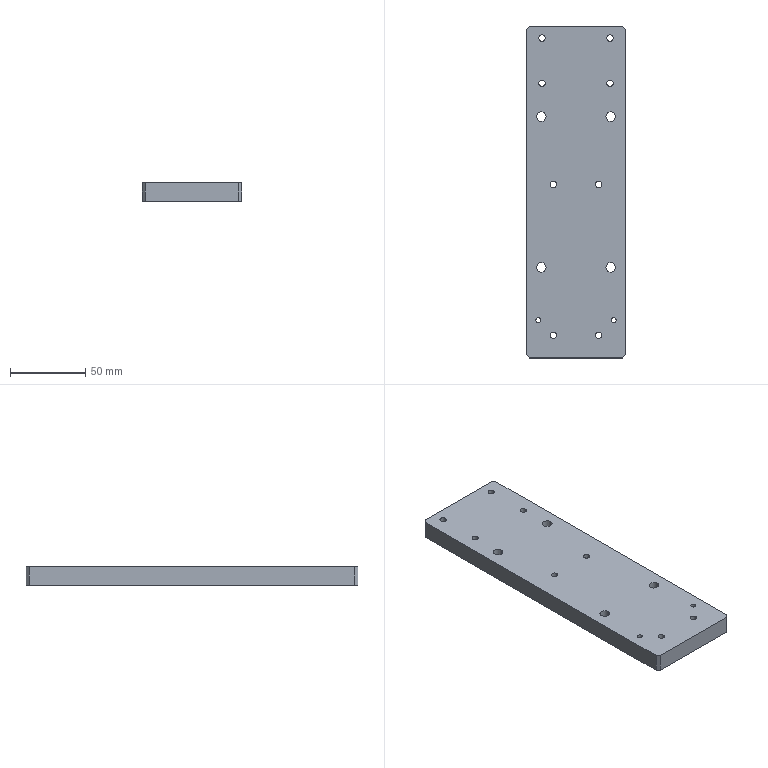Part | STEP file | 1 solid | 50 faces | box 66 x 220 x 12 mm | volume 169355 mm3 | cylinder 36 | plane 14 | commonest cylinder face diameters 4.2 x16 6.4 x8 11 x8 3.3 x4